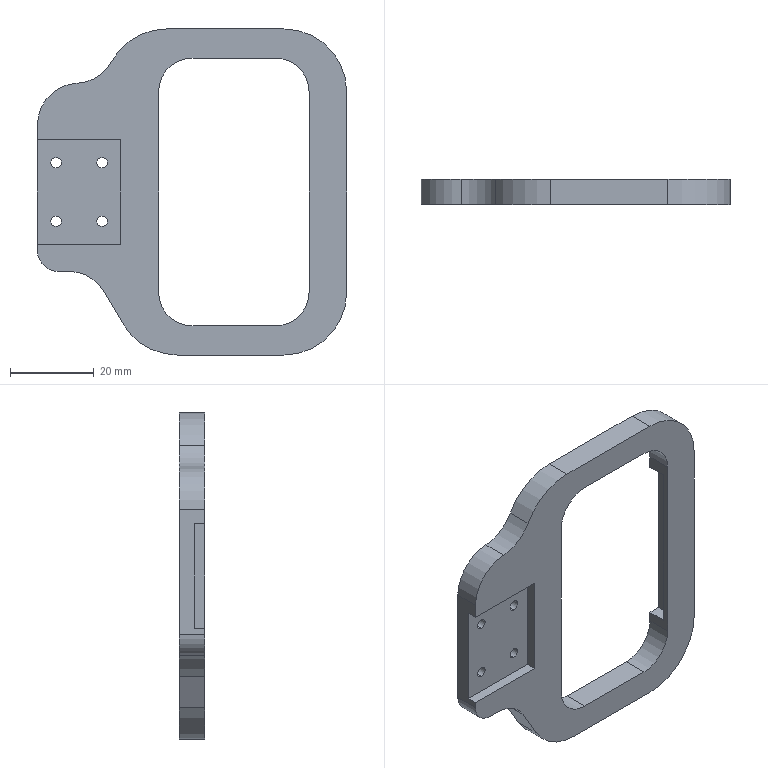Part | SolidWorks | features BaseBody 1, Cut 1, HoleWzd 1 | 1 solid | 44 faces | box 74 x 6 x 78 mm | volume 14123 mm3 | plane 24 | cylinder 20 | commonest cylinder face diameters 2.5 x8 16 x4 30 x4 20 x3 10 x1
STEP:
#1=CARTESIAN_POINT('',(1280.5,6.,-8.25));
#2=VERTEX_POINT('',#1);
#3=CARTESIAN_POINT('',(1280.5,6.,-5.75));
#4=VERTEX_POINT('',#3);
#5=CARTESIAN_POINT('',(1280.5,6.,-7.));
#6=DIRECTION('',(0.,1.,0.));
#7=DIRECTION('',(0.,0.,1.));
#8=AXIS2_PLACEMENT_3D('',#5,#6,#7);
#9=CIRCLE('',#8,1.25);
#10=EDGE_CURVE('',#2,#4,#9,.T.);
#11=ORIENTED_EDGE('',*,*,#10,.T.);
#12=CARTESIAN_POINT('',(1280.5,2.5,-5.75));
#13=VERTEX_POINT('',#12);
#14=CARTESIAN_POINT('',(1280.5,0.,-5.75));
#15=DIRECTION('',(0.,-1.,0.));
#16=VECTOR('',#15,1000.);
#17=LINE('',#14,#16);
#18=EDGE_CURVE('',#4,#13,#17,.T.);
#19=ORIENTED_EDGE('',*,*,#18,.T.);
#20=CARTESIAN_POINT('',(1280.5,2.5,-8.25));
#21=VERTEX_POINT('',#20);
#22=CARTESIAN_POINT('',(1280.5,2.5,-7.));
#23=DIRECTION('',(0.,-1.,0.));
#24=DIRECTION('',(0.,0.,-1.));
#25=AXIS2_PLACEMENT_3D('',#22,#23,#24);
#26=CIRCLE('',#25,1.25);
#27=EDGE_CURVE('',#13,#21,#26,.T.);
#28=ORIENTED_EDGE('',*,*,#27,.T.);
#29=CARTESIAN_POINT('',(1280.5,0.,-8.25));
#30=DIRECTION('',(0.,-1.,0.));
#31=VECTOR('',#30,1000.);
#32=LINE('',#29,#31);
#33=EDGE_CURVE('',#2,#21,#32,.T.);
#34=ORIENTED_EDGE('',*,*,#33,.F.);
#35=EDGE_LOOP('',(#11,#19,#28,#34));
#36=FACE_OUTER_BOUND('',#35,.T.);
#37=CARTESIAN_POINT('',(1280.5,0.,-7.));
#38=DIRECTION('',(0.,-1.,0.));
#39=DIRECTION('',(0.,0.,-1.));
#40=AXIS2_PLACEMENT_3D('',#37,#38,#39);
#41=CYLINDRICAL_SURFACE('',#40,1.25);
#42=ADVANCED_FACE('',(#36),#41,.F.);
#43=CARTESIAN_POINT('',(1269.5,6.,-8.25));
#44=VERTEX_POINT('',#43);
#45=CARTESIAN_POINT('',(1269.5,6.,-5.75));
#46=VERTEX_POINT('',#45);
#47=CARTESIAN_POINT('',(1269.5,6.,-7.));
#48=DIRECTION('',(0.,1.,0.));
#49=DIRECTION('',(0.,0.,1.));
#50=AXIS2_PLACEMENT_3D('',#47,#48,#49);
#51=CIRCLE('',#50,1.25);
#52=EDGE_CURVE('',#44,#46,#51,.T.);
#53=ORIENTED_EDGE('',*,*,#52,.T.);
#54=CARTESIAN_POINT('',(1269.5,2.5,-5.75));
#55=VERTEX_POINT('',#54);
#56=CARTESIAN_POINT('',(1269.5,0.,-5.75));
#57=DIRECTION('',(0.,-1.,0.));
#58=VECTOR('',#57,1000.);
#59=LINE('',#56,#58);
#60=EDGE_CURVE('',#46,#55,#59,.T.);
#61=ORIENTED_EDGE('',*,*,#60,.T.);
#62=CARTESIAN_POINT('',(1269.5,2.5,-8.25));
#63=VERTEX_POINT('',#62);
#64=CARTESIAN_POINT('',(1269.5,2.5,-7.));
#65=DIRECTION('',(0.,-1.,0.));
#66=DIRECTION('',(0.,0.,-1.));
#67=AXIS2_PLACEMENT_3D('',#64,#65,#66);
#68=CIRCLE('',#67,1.25);
#69=EDGE_CURVE('',#55,#63,#68,.T.);
#70=ORIENTED_EDGE('',*,*,#69,.T.);
#71=CARTESIAN_POINT('',(1269.5,0.,-8.25));
#72=DIRECTION('',(0.,-1.,0.));
#73=VECTOR('',#72,1000.);
#74=LINE('',#71,#73);
#75=EDGE_CURVE('',#44,#63,#74,.T.);
#76=ORIENTED_EDGE('',*,*,#75,.F.);
#77=EDGE_LOOP('',(#53,#61,#70,#76));
#78=FACE_OUTER_BOUND('',#77,.T.);
#79=CARTESIAN_POINT('',(1269.5,0.,-7.));
#80=DIRECTION('',(0.,-1.,0.));
#81=DIRECTION('',(0.,0.,-1.));
#82=AXIS2_PLACEMENT_3D('',#79,#80,#81);
#83=CYLINDRICAL_SURFACE('',#82,1.25);
#84=ADVANCED_FACE('',(#78),#83,.F.);
#85=CARTESIAN_POINT('',(1269.5,6.,5.75));
#86=VERTEX_POINT('',#85);
#87=CARTESIAN_POINT('',(1269.5,6.,8.25));
#88=VERTEX_POINT('',#87);
#89=CARTESIAN_POINT('',(1269.5,6.,7.));
#90=DIRECTION('',(0.,1.,0.));
#91=DIRECTION('',(0.,0.,1.));
#92=AXIS2_PLACEMENT_3D('',#89,#90,#91);
#93=CIRCLE('',#92,1.25);
#94=EDGE_CURVE('',#86,#88,#93,.T.);
#95=ORIENTED_EDGE('',*,*,#94,.T.);
#96=CARTESIAN_POINT('',(1269.5,2.5,8.25));
#97=VERTEX_POINT('',#96);
#98=CARTESIAN_POINT('',(1269.5,0.,8.25));
#99=DIRECTION('',(0.,-1.,0.));
#100=VECTOR('',#99,1000.);
#101=LINE('',#98,#100);
#102=EDGE_CURVE('',#88,#97,#101,.T.);
#103=ORIENTED_EDGE('',*,*,#102,.T.);
#104=CARTESIAN_POINT('',(1269.5,2.5,5.75));
#105=VERTEX_POINT('',#104);
#106=CARTESIAN_POINT('',(1269.5,2.5,7.));
#107=DIRECTION('',(0.,-1.,0.));
#108=DIRECTION('',(0.,0.,-1.));
#109=AXIS2_PLACEMENT_3D('',#106,#107,#108);
#110=CIRCLE('',#109,1.25);
#111=EDGE_CURVE('',#97,#105,#110,.T.);
#112=ORIENTED_EDGE('',*,*,#111,.T.);
#113=CARTESIAN_POINT('',(1269.5,0.,5.75));
#114=DIRECTION('',(0.,-1.,0.));
#115=VECTOR('',#114,1000.);
#116=LINE('',#113,#115);
#117=EDGE_CURVE('',#86,#105,#116,.T.);
#118=ORIENTED_EDGE('',*,*,#117,.F.);
#119=EDGE_LOOP('',(#95,#103,#112,#118));
#120=FACE_OUTER_BOUND('',#119,.T.);
#121=CARTESIAN_POINT('',(1269.5,0.,7.));
#122=DIRECTION('',(0.,-1.,0.));
#123=DIRECTION('',(0.,0.,-1.));
#124=AXIS2_PLACEMENT_3D('',#121,#122,#123);
#125=CYLINDRICAL_SURFACE('',#124,1.25);
#126=ADVANCED_FACE('',(#120),#125,.F.);
#127=CARTESIAN_POINT('',(1280.5,6.,5.75));
#128=VERTEX_POINT('',#127);
#129=CARTESIAN_POINT('',(1280.5,6.,8.25));
#130=VERTEX_POINT('',#129);
#131=CARTESIAN_POINT('',(1280.5,6.,7.));
#132=DIRECTION('',(0.,1.,0.));
#133=DIRECTION('',(0.,0.,1.));
#134=AXIS2_PLACEMENT_3D('',#131,#132,#133);
#135=CIRCLE('',#134,1.25);
#136=EDGE_CURVE('',#128,#130,#135,.T.);
#137=ORIENTED_EDGE('',*,*,#136,.T.);
#138=CARTESIAN_POINT('',(1280.5,2.5,8.25));
#139=VERTEX_POINT('',#138);
#140=CARTESIAN_POINT('',(1280.5,0.,8.25));
#141=DIRECTION('',(0.,-1.,0.));
#142=VECTOR('',#141,1000.);
#143=LINE('',#140,#142);
#144=EDGE_CURVE('',#130,#139,#143,.T.);
#145=ORIENTED_EDGE('',*,*,#144,.T.);
#146=CARTESIAN_POINT('',(1280.5,2.5,5.75));
#147=VERTEX_POINT('',#146);
#148=CARTESIAN_POINT('',(1280.5,2.5,7.));
#149=DIRECTION('',(0.,-1.,0.));
#150=DIRECTION('',(0.,0.,-1.));
#151=AXIS2_PLACEMENT_3D('',#148,#149,#150);
#152=CIRCLE('',#151,1.25);
#153=EDGE_CURVE('',#139,#147,#152,.T.);
#154=ORIENTED_EDGE('',*,*,#153,.T.);
#155=CARTESIAN_POINT('',(1280.5,0.,5.75));
#156=DIRECTION('',(0.,-1.,0.));
#157=VECTOR('',#156,1000.);
#158=LINE('',#155,#157);
#159=EDGE_CURVE('',#128,#147,#158,.T.);
#160=ORIENTED_EDGE('',*,*,#159,.F.);
#161=EDGE_LOOP('',(#137,#145,#154,#160));
#162=FACE_OUTER_BOUND('',#161,.T.);
#163=CARTESIAN_POINT('',(1280.5,0.,7.));
#164=DIRECTION('',(0.,-1.,0.));
#165=DIRECTION('',(0.,0.,-1.));
#166=AXIS2_PLACEMENT_3D('',#163,#164,#165);
#167=CYLINDRICAL_SURFACE('',#166,1.25);
#168=ADVANCED_FACE('',(#162),#167,.F.);
#169=CARTESIAN_POINT('',(1285.,0.,12.5));
#170=VERTEX_POINT('',#169);
#171=CARTESIAN_POINT('',(1265.,0.,12.5));
#172=VERTEX_POINT('',#171);
#173=CARTESIAN_POINT('',(1265.,0.,12.5));
#174=DIRECTION('',(-1.,0.,0.));
#175=VECTOR('',#174,1000.);
#176=LINE('',#173,#175);
#177=EDGE_CURVE('',#170,#172,#176,.T.);
#178=ORIENTED_EDGE('',*,*,#177,.F.);
#179=CARTESIAN_POINT('',(1285.,0.,-12.5));
#180=VERTEX_POINT('',#179);
#181=CARTESIAN_POINT('',(1285.,0.,12.5));
#182=DIRECTION('',(0.,0.,1.));
#183=VECTOR('',#182,1000.);
#184=LINE('',#181,#183);
#185=EDGE_CURVE('',#180,#170,#184,.T.);
#186=ORIENTED_EDGE('',*,*,#185,.F.);
#187=CARTESIAN_POINT('',(1265.,0.,-12.5));
#188=VERTEX_POINT('',#187);
#189=CARTESIAN_POINT('',(1265.,0.,-12.5));
#190=DIRECTION('',(1.,0.,0.));
#191=VECTOR('',#190,1000.);
#192=LINE('',#189,#191);
#193=EDGE_CURVE('',#188,#180,#192,.T.);
#194=ORIENTED_EDGE('',*,*,#193,.F.);
#195=CARTESIAN_POINT('',(1265.,0.,-13.995));
#196=VERTEX_POINT('',#195);
#197=CARTESIAN_POINT('',(1265.,0.,0.));
#198=DIRECTION('',(0.,0.,-1.));
#199=VECTOR('',#198,1000.);
#200=LINE('',#197,#199);
#201=EDGE_CURVE('',#188,#196,#200,.T.);
#202=ORIENTED_EDGE('',*,*,#201,.T.);
#203=CARTESIAN_POINT('',(1270.,0.,-18.995));
#204=VERTEX_POINT('',#203);
#205=CARTESIAN_POINT('',(1270.,0.,-13.995));
#206=DIRECTION('',(0.,-1.,0.));
#207=DIRECTION('',(0.,0.,-1.));
#208=AXIS2_PLACEMENT_3D('',#205,#206,#207);
#209=CIRCLE('',#208,5.);
#210=EDGE_CURVE('',#196,#204,#209,.T.);
#211=ORIENTED_EDGE('',*,*,#210,.T.);
#212=CARTESIAN_POINT('',(1272.447,0.,-18.995));
#213=VERTEX_POINT('',#212);
#214=CARTESIAN_POINT('',(0.,0.,-18.995));
#215=DIRECTION('',(1.,0.,0.));
#216=VECTOR('',#215,1000.);
#217=LINE('',#214,#216);
#218=EDGE_CURVE('',#204,#213,#217,.T.);
#219=ORIENTED_EDGE('',*,*,#218,.T.);
#220=CARTESIAN_POINT('',(1281.087,0.,-23.96));
#221=VERTEX_POINT('',#220);
#222=CARTESIAN_POINT('',(1272.447,0.,-28.995));
#223=DIRECTION('',(0.,1.,0.));
#224=DIRECTION('',(0.,0.,1.));
#225=AXIS2_PLACEMENT_3D('',#222,#223,#224);
#226=CIRCLE('',#225,10.);
#227=EDGE_CURVE('',#213,#221,#226,.T.);
#228=ORIENTED_EDGE('',*,*,#227,.T.);
#229=CARTESIAN_POINT('',(1285.513,0.,-31.554));
#230=VERTEX_POINT('',#229);
#231=CARTESIAN_POINT('',(1281.087,0.,-23.96));
#232=DIRECTION('',(0.5036,0.,-0.8639));
#233=VECTOR('',#232,1000.);
#234=LINE('',#231,#233);
#235=EDGE_CURVE('',#221,#230,#234,.T.);
#236=ORIENTED_EDGE('',*,*,#235,.T.);
#237=CARTESIAN_POINT('',(1298.473,0.,-39.));
#238=VERTEX_POINT('',#237);
#239=CARTESIAN_POINT('',(1298.473,0.,-24.));
#240=DIRECTION('',(0.,-1.,0.));
#241=DIRECTION('',(0.,0.,1.));
#242=AXIS2_PLACEMENT_3D('',#239,#240,#241);
#243=CIRCLE('',#242,15.);
#244=EDGE_CURVE('',#230,#238,#243,.T.);
#245=ORIENTED_EDGE('',*,*,#244,.T.);
#246=CARTESIAN_POINT('',(1324.,0.,-39.));
#247=VERTEX_POINT('',#246);
#248=CARTESIAN_POINT('',(0.,0.,-39.));
#249=DIRECTION('',(1.,0.,0.));
#250=VECTOR('',#249,1000.);
#251=LINE('',#248,#250);
#252=EDGE_CURVE('',#238,#247,#251,.T.);
#253=ORIENTED_EDGE('',*,*,#252,.T.);
#254=CARTESIAN_POINT('',(1339.,0.,-24.));
#255=VERTEX_POINT('',#254);
#256=CARTESIAN_POINT('',(1324.,0.,-24.));
#257=DIRECTION('',(0.,-1.,0.));
#258=DIRECTION('',(0.,0.,1.));
#259=AXIS2_PLACEMENT_3D('',#256,#257,#258);
#260=CIRCLE('',#259,15.);
#261=EDGE_CURVE('',#247,#255,#260,.T.);
#262=ORIENTED_EDGE('',*,*,#261,.T.);
#263=CARTESIAN_POINT('',(1339.,0.,24.));
#264=VERTEX_POINT('',#263);
#265=CARTESIAN_POINT('',(1339.,0.,0.));
#266=DIRECTION('',(0.,0.,1.));
#267=VECTOR('',#266,1000.);
#268=LINE('',#265,#267);
#269=EDGE_CURVE('',#255,#264,#268,.T.);
#270=ORIENTED_EDGE('',*,*,#269,.T.);
#271=CARTESIAN_POINT('',(1324.,0.,39.));
#272=VERTEX_POINT('',#271);
#273=CARTESIAN_POINT('',(1324.,0.,24.));
#274=DIRECTION('',(0.,-1.,0.));
#275=DIRECTION('',(0.,0.,1.));
#276=AXIS2_PLACEMENT_3D('',#273,#274,#275);
#277=CIRCLE('',#276,15.);
#278=EDGE_CURVE('',#264,#272,#277,.T.);
#279=ORIENTED_EDGE('',*,*,#278,.T.);
#280=CARTESIAN_POINT('',(1295.928,0.,39.));
#281=VERTEX_POINT('',#280);
#282=CARTESIAN_POINT('',(0.,0.,39.));
#283=DIRECTION('',(-1.,0.,0.));
#284=VECTOR('',#283,1000.);
#285=LINE('',#282,#284);
#286=EDGE_CURVE('',#272,#281,#285,.T.);
#287=ORIENTED_EDGE('',*,*,#286,.T.);
#288=CARTESIAN_POINT('',(1282.769,0.,31.2));
#289=VERTEX_POINT('',#288);
#290=CARTESIAN_POINT('',(1295.928,0.,24.));
#291=DIRECTION('',(0.,-1.,0.));
#292=DIRECTION('',(0.,0.,1.));
#293=AXIS2_PLACEMENT_3D('',#290,#291,#292);
#294=CIRCLE('',#293,15.);
#295=EDGE_CURVE('',#281,#289,#294,.T.);
#296=ORIENTED_EDGE('',*,*,#295,.T.);
#297=CARTESIAN_POINT('',(1274.498,0.,26.013));
#298=VERTEX_POINT('',#297);
#299=CARTESIAN_POINT('',(1273.997,0.,36.));
#300=DIRECTION('',(0.,1.,0.));
#301=DIRECTION('',(0.,0.,1.));
#302=AXIS2_PLACEMENT_3D('',#299,#300,#301);
#303=CIRCLE('',#302,10.);
#304=EDGE_CURVE('',#289,#298,#303,.T.);
#305=ORIENTED_EDGE('',*,*,#304,.T.);
#306=CARTESIAN_POINT('',(1265.,0.,16.025));
#307=VERTEX_POINT('',#306);
#308=CARTESIAN_POINT('',(1275.,0.,16.025));
#309=DIRECTION('',(0.,-1.,0.));
#310=DIRECTION('',(0.,0.,-1.));
#311=AXIS2_PLACEMENT_3D('',#308,#309,#310);
#312=CIRCLE('',#311,10.);
#313=EDGE_CURVE('',#298,#307,#312,.T.);
#314=ORIENTED_EDGE('',*,*,#313,.T.);
#315=CARTESIAN_POINT('',(1265.,0.,0.));
#316=DIRECTION('',(0.,0.,-1.));
#317=VECTOR('',#316,1000.);
#318=LINE('',#315,#317);
#319=EDGE_CURVE('',#307,#172,#318,.T.);
#320=ORIENTED_EDGE('',*,*,#319,.T.);
#321=EDGE_LOOP('',(#178,#186,#194,#202,#211,#219,#228,#236,#245,#253,#262,#270,#279,#287,#296,#305,#314,#320));
#322=FACE_OUTER_BOUND('',#321,.T.);
#323=CARTESIAN_POINT('',(1330.,0.,-24.));
#324=VERTEX_POINT('',#323);
#325=CARTESIAN_POINT('',(1322.,0.,-32.));
#326=VERTEX_POINT('',#325);
#327=CARTESIAN_POINT('',(1322.,0.,-24.));
#328=DIRECTION('',(0.,1.,0.));
#329=DIRECTION('',(0.,0.,1.));
#330=AXIS2_PLACEMENT_3D('',#327,#328,#329);
#331=CIRCLE('',#330,8.);
#332=EDGE_CURVE('',#324,#326,#331,.T.);
#333=ORIENTED_EDGE('',*,*,#332,.T.);
#334=CARTESIAN_POINT('',(1302.,0.,-32.));
#335=VERTEX_POINT('',#334);
#336=CARTESIAN_POINT('',(0.,0.,-32.));
#337=DIRECTION('',(-1.,0.,0.));
#338=VECTOR('',#337,1000.);
#339=LINE('',#336,#338);
#340=EDGE_CURVE('',#326,#335,#339,.T.);
#341=ORIENTED_EDGE('',*,*,#340,.T.);
#342=CARTESIAN_POINT('',(1294.,0.,-24.));
#343=VERTEX_POINT('',#342);
#344=CARTESIAN_POINT('',(1302.,0.,-24.));
#345=DIRECTION('',(0.,1.,0.));
#346=DIRECTION('',(0.,0.,1.));
#347=AXIS2_PLACEMENT_3D('',#344,#345,#346);
#348=CIRCLE('',#347,8.);
#349=EDGE_CURVE('',#335,#343,#348,.T.);
#350=ORIENTED_EDGE('',*,*,#349,.T.);
#351=CARTESIAN_POINT('',(1294.,0.,24.));
#352=VERTEX_POINT('',#351);
#353=CARTESIAN_POINT('',(1294.,0.,0.));
#354=DIRECTION('',(0.,0.,1.));
#355=VECTOR('',#354,1000.);
#356=LINE('',#353,#355);
#357=EDGE_CURVE('',#343,#352,#356,.T.);
#358=ORIENTED_EDGE('',*,*,#357,.T.);
#359=CARTESIAN_POINT('',(1302.,0.,32.));
#360=VERTEX_POINT('',#359);
#361=CARTESIAN_POINT('',(1302.,0.,24.));
#362=DIRECTION('',(0.,1.,0.));
#363=DIRECTION('',(0.,0.,1.));
#364=AXIS2_PLACEMENT_3D('',#361,#362,#363);
#365=CIRCLE('',#364,8.);
#366=EDGE_CURVE('',#352,#360,#365,.T.);
#367=ORIENTED_EDGE('',*,*,#366,.T.);
#368=CARTESIAN_POINT('',(1322.,0.,32.));
#369=VERTEX_POINT('',#368);
#370=CARTESIAN_POINT('',(0.,0.,32.));
#371=DIRECTION('',(1.,0.,0.));
#372=VECTOR('',#371,1000.);
#373=LINE('',#370,#372);
#374=EDGE_CURVE('',#360,#369,#373,.T.);
#375=ORIENTED_EDGE('',*,*,#374,.T.);
#376=CARTESIAN_POINT('',(1330.,0.,24.));
#377=VERTEX_POINT('',#376);
#378=CARTESIAN_POINT('',(1322.,0.,24.));
#379=DIRECTION('',(0.,1.,0.));
#380=DIRECTION('',(0.,0.,1.));
#381=AXIS2_PLACEMENT_3D('',#378,#379,#380);
#382=CIRCLE('',#381,8.);
#383=EDGE_CURVE('',#369,#377,#382,.T.);
#384=ORIENTED_EDGE('',*,*,#383,.T.);
#385=CARTESIAN_POINT('',(1330.,0.,0.));
#386=DIRECTION('',(0.,0.,-1.));
#387=VECTOR('',#386,1000.);
#388=LINE('',#385,#387);
#389=EDGE_CURVE('',#377,#324,#388,.T.);
#390=ORIENTED_EDGE('',*,*,#389,.T.);
#391=EDGE_LOOP('',(#333,#341,#350,#358,#367,#375,#384,#390));
#392=FACE_BOUND('',#391,.T.);
#393=CARTESIAN_POINT('',(0.,0.,0.));
#394=DIRECTION('',(0.,-1.,0.));
#395=DIRECTION('',(0.,0.,-1.));
#396=AXIS2_PLACEMENT_3D('',#393,#394,#395);
#397=PLANE('',#396);
#398=ADVANCED_FACE('',(#322,#392),#397,.T.);
#399=CARTESIAN_POINT('',(1302.,6.,-32.));
#400=VERTEX_POINT('',#399);
#401=CARTESIAN_POINT('',(1322.,6.,-32.));
#402=VERTEX_POINT('',#401);
#403=CARTESIAN_POINT('',(1302.,6.,-32.));
#404=DIRECTION('',(1.,0.,0.));
#405=VECTOR('',#404,1000.);
#406=LINE('',#403,#405);
#407=EDGE_CURVE('',#400,#402,#406,.T.);
#408=ORIENTED_EDGE('',*,*,#407,.F.);
#409=CARTESIAN_POINT('',(1302.,0.,-32.));
#410=DIRECTION('',(0.,1.,0.));
#411=VECTOR('',#410,1000.);
#412=LINE('',#409,#411);
#413=EDGE_CURVE('',#335,#400,#412,.T.);
#414=ORIENTED_EDGE('',*,*,#413,.F.);
#415=ORIENTED_EDGE('',*,*,#340,.F.);
#416=CARTESIAN_POINT('',(1322.,0.,-32.));
#417=DIRECTION('',(0.,-1.,0.));
#418=VECTOR('',#417,1000.);
#419=LINE('',#416,#418);
#420=EDGE_CURVE('',#402,#326,#419,.T.);
#421=ORIENTED_EDGE('',*,*,#420,.F.);
#422=EDGE_LOOP('',(#408,#414,#415,#421));
#423=FACE_OUTER_BOUND('',#422,.T.);
#424=CARTESIAN_POINT('',(1302.,0.,-32.));
#425=DIRECTION('',(0.,0.,-1.));
#426=DIRECTION('',(-1.,0.,0.));
#427=AXIS2_PLACEMENT_3D('',#424,#425,#426);
#428=PLANE('',#427);
#429=ADVANCED_FACE('',(#423),#428,.F.);
#430=CARTESIAN_POINT('',(1330.,6.,-24.));
#431=VERTEX_POINT('',#430);
#432=CARTESIAN_POINT('',(1322.,6.,-24.));
#433=DIRECTION('',(0.,-1.,0.));
#434=DIRECTION('',(0.,0.,1.));
#435=AXIS2_PLACEMENT_3D('',#432,#433,#434);
#436=CIRCLE('',#435,8.);
#437=EDGE_CURVE('',#402,#431,#436,.T.);
#438=ORIENTED_EDGE('',*,*,#437,.F.);
#439=ORIENTED_EDGE('',*,*,#420,.T.);
#440=ORIENTED_EDGE('',*,*,#332,.F.);
#441=CARTESIAN_POINT('',(1330.,0.,-24.));
#442=DIRECTION('',(0.,-1.,0.));
#443=VECTOR('',#442,1000.);
#444=LINE('',#441,#443);
#445=EDGE_CURVE('',#431,#324,#444,.T.);
#446=ORIENTED_EDGE('',*,*,#445,.F.);
#447=EDGE_LOOP('',(#438,#439,#440,#446));
#448=FACE_OUTER_BOUND('',#447,.T.);
#449=CARTESIAN_POINT('',(1322.,0.,-24.));
#450=DIRECTION('',(0.,1.,0.));
#451=DIRECTION('',(0.,0.,1.));
#452=AXIS2_PLACEMENT_3D('',#449,#450,#451);
#453=CYLINDRICAL_SURFACE('',#452,8.);
#454=ADVANCED_FACE('',(#448),#453,.F.);
#455=CARTESIAN_POINT('',(1330.,6.,-21.548));
#456=VERTEX_POINT('',#455);
#457=CARTESIAN_POINT('',(1330.,6.,-24.));
#458=DIRECTION('',(0.,0.,1.));
#459=VECTOR('',#458,1000.);
#460=LINE('',#457,#459);
#461=EDGE_CURVE('',#431,#456,#460,.T.);
#462=ORIENTED_EDGE('',*,*,#461,.F.);
#463=ORIENTED_EDGE('',*,*,#445,.T.);
#464=ORIENTED_EDGE('',*,*,#389,.F.);
#465=CARTESIAN_POINT('',(1330.,6.,24.));
#466=VERTEX_POINT('',#465);
#467=CARTESIAN_POINT('',(1330.,0.,24.));
#468=DIRECTION('',(0.,-1.,0.));
#469=VECTOR('',#468,1000.);
#470=LINE('',#467,#469);
#471=EDGE_CURVE('',#466,#377,#470,.T.);
#472=ORIENTED_EDGE('',*,*,#471,.F.);
#473=CARTESIAN_POINT('',(1330.,6.,21.019));
#474=VERTEX_POINT('',#473);
#475=CARTESIAN_POINT('',(1330.,6.,-24.));
#476=DIRECTION('',(0.,0.,1.));
#477=VECTOR('',#476,1000.);
#478=LINE('',#475,#477);
#479=EDGE_CURVE('',#474,#466,#478,.T.);
#480=ORIENTED_EDGE('',*,*,#479,.F.);
#481=CARTESIAN_POINT('',(1330.,1.5,21.019));
#482=VERTEX_POINT('',#481);
#483=CARTESIAN_POINT('',(1330.,0.,21.019));
#484=DIRECTION('',(0.,1.,0.));
#485=VECTOR('',#484,1000.);
#486=LINE('',#483,#485);
#487=EDGE_CURVE('',#482,#474,#486,.T.);
#488=ORIENTED_EDGE('',*,*,#487,.F.);
#489=CARTESIAN_POINT('',(1330.,1.5,-21.548));
#490=VERTEX_POINT('',#489);
#491=CARTESIAN_POINT('',(1330.,1.5,-24.));
#492=DIRECTION('',(0.,0.,1.));
#493=VECTOR('',#492,1000.);
#494=LINE('',#491,#493);
#495=EDGE_CURVE('',#490,#482,#494,.T.);
#496=ORIENTED_EDGE('',*,*,#495,.F.);
#497=CARTESIAN_POINT('',(1330.,0.,-21.548));
#498=DIRECTION('',(0.,-1.,0.));
#499=VECTOR('',#498,1000.);
#500=LINE('',#497,#499);
#501=EDGE_CURVE('',#456,#490,#500,.T.);
#502=ORIENTED_EDGE('',*,*,#501,.F.);
#503=EDGE_LOOP('',(#462,#463,#464,#472,#480,#488,#496,#502));
#504=FACE_OUTER_BOUND('',#503,.T.);
#505=CARTESIAN_POINT('',(1330.,0.,-24.));
#506=DIRECTION('',(1.,0.,0.));
#507=DIRECTION('',(0.,0.,-1.));
#508=AXIS2_PLACEMENT_3D('',#505,#506,#507);
#509=PLANE('',#508);
#510=ADVANCED_FACE('',(#504),#509,.F.);
#511=CARTESIAN_POINT('',(1322.,6.,32.));
#512=VERTEX_POINT('',#511);
#513=CARTESIAN_POINT('',(1322.,6.,24.));
#514=DIRECTION('',(0.,-1.,0.));
#515=DIRECTION('',(0.,0.,1.));
#516=AXIS2_PLACEMENT_3D('',#513,#514,#515);
#517=CIRCLE('',#516,8.);
#518=EDGE_CURVE('',#466,#512,#517,.T.);
#519=ORIENTED_EDGE('',*,*,#518,.F.);
#520=ORIENTED_EDGE('',*,*,#471,.T.);
#521=ORIENTED_EDGE('',*,*,#383,.F.);
#522=CARTESIAN_POINT('',(1322.,0.,32.));
#523=DIRECTION('',(0.,-1.,0.));
#524=VECTOR('',#523,1000.);
#525=LINE('',#522,#524);
#526=EDGE_CURVE('',#512,#369,#525,.T.);
#527=ORIENTED_EDGE('',*,*,#526,.F.);
#528=EDGE_LOOP('',(#519,#520,#521,#527));
#529=FACE_OUTER_BOUND('',#528,.T.);
#530=CARTESIAN_POINT('',(1322.,0.,24.));
#531=DIRECTION('',(0.,1.,0.));
#532=DIRECTION('',(0.,0.,1.));
#533=AXIS2_PLACEMENT_3D('',#530,#531,#532);
#534=CYLINDRICAL_SURFACE('',#533,8.);
#535=ADVANCED_FACE('',(#529),#534,.F.);
#536=CARTESIAN_POINT('',(1302.,6.,32.));
#537=VERTEX_POINT('',#536);
#538=CARTESIAN_POINT('',(1322.,6.,32.));
#539=DIRECTION('',(-1.,0.,0.));
#540=VECTOR('',#539,1000.);
#541=LINE('',#538,#540);
#542=EDGE_CURVE('',#512,#537,#541,.T.);
#543=ORIENTED_EDGE('',*,*,#542,.F.);
#544=ORIENTED_EDGE('',*,*,#526,.T.);
#545=ORIENTED_EDGE('',*,*,#374,.F.);
#546=CARTESIAN_POINT('',(1302.,0.,32.));
#547=DIRECTION('',(0.,-1.,0.));
#548=VECTOR('',#547,1000.);
#549=LINE('',#546,#548);
#550=EDGE_CURVE('',#537,#360,#549,.T.);
#551=ORIENTED_EDGE('',*,*,#550,.F.);
#552=EDGE_LOOP('',(#543,#544,#545,#551));
#553=FACE_OUTER_BOUND('',#552,.T.);
#554=CARTESIAN_POINT('',(1322.,0.,32.));
#555=DIRECTION('',(0.,0.,1.));
#556=DIRECTION('',(1.,0.,0.));
#557=AXIS2_PLACEMENT_3D('',#554,#555,#556);
#558=PLANE('',#557);
#559=ADVANCED_FACE('',(#553),#558,.F.);
#560=CARTESIAN_POINT('',(1294.,6.,24.));
#561=VERTEX_POINT('',#560);
#562=CARTESIAN_POINT('',(1302.,6.,24.));
#563=DIRECTION('',(0.,-1.,0.));
#564=DIRECTION('',(0.,0.,1.));
#565=AXIS2_PLACEMENT_3D('',#562,#563,#564);
#566=CIRCLE('',#565,8.);
#567=EDGE_CURVE('',#537,#561,#566,.T.);
#568=ORIENTED_EDGE('',*,*,#567,.F.);
#569=ORIENTED_EDGE('',*,*,#550,.T.);
#570=ORIENTED_EDGE('',*,*,#366,.F.);
#571=CARTESIAN_POINT('',(1294.,0.,24.));
#572=DIRECTION('',(0.,-1.,0.));
#573=VECTOR('',#572,1000.);
#574=LINE('',#571,#573);
#575=EDGE_CURVE('',#561,#352,#574,.T.);
#576=ORIENTED_EDGE('',*,*,#575,.F.);
#577=EDGE_LOOP('',(#568,#569,#570,#576));
#578=FACE_OUTER_BOUND('',#577,.T.);
#579=CARTESIAN_POINT('',(1302.,0.,24.));
#580=DIRECTION('',(0.,1.,0.));
#581=DIRECTION('',(0.,0.,1.));
#582=AXIS2_PLACEMENT_3D('',#579,#580,#581);
#583=CYLINDRICAL_SURFACE('',#582,8.);
#584=ADVANCED_FACE('',(#578),#583,.F.);
#585=CARTESIAN_POINT('',(1294.,6.,21.019));
#586=VERTEX_POINT('',#585);
#587=CARTESIAN_POINT('',(1294.,6.,24.));
#588=DIRECTION('',(0.,0.,-1.));
#589=VECTOR('',#588,1000.);
#590=LINE('',#587,#589);
#591=EDGE_CURVE('',#561,#586,#590,.T.);
#592=ORIENTED_EDGE('',*,*,#591,.F.);
#593=ORIENTED_EDGE('',*,*,#575,.T.);
#594=ORIENTED_EDGE('',*,*,#357,.F.);
#595=CARTESIAN_POINT('',(1294.,6.,-24.));
#596=VERTEX_POINT('',#595);
#597=CARTESIAN_POINT('',(1294.,0.,-24.));
#598=DIRECTION('',(0.,-1.,0.));
#599=VECTOR('',#598,1000.);
#600=LINE('',#597,#599);
#601=EDGE_CURVE('',#596,#343,#600,.T.);
#602=ORIENTED_EDGE('',*,*,#601,.F.);
#603=CARTESIAN_POINT('',(1294.,6.,-21.548));
#604=VERTEX_POINT('',#603);
#605=CARTESIAN_POINT('',(1294.,6.,24.));
#606=DIRECTION('',(0.,0.,-1.));
#607=VECTOR('',#606,1000.);
#608=LINE('',#605,#607);
#609=EDGE_CURVE('',#604,#596,#608,.T.);
#610=ORIENTED_EDGE('',*,*,#609,.F.);
#611=CARTESIAN_POINT('',(1294.,1.5,-21.548));
#612=VERTEX_POINT('',#611);
#613=CARTESIAN_POINT('',(1294.,0.,-21.548));
#614=DIRECTION('',(0.,1.,0.));
#615=VECTOR('',#614,1000.);
#616=LINE('',#613,#615);
#617=EDGE_CURVE('',#612,#604,#616,.T.);
#618=ORIENTED_EDGE('',*,*,#617,.F.);
#619=CARTESIAN_POINT('',(1294.,1.5,21.019));
#620=VERTEX_POINT('',#619);
#621=CARTESIAN_POINT('',(1294.,1.5,24.));
#622=DIRECTION('',(0.,0.,-1.));
#623=VECTOR('',#622,1000.);
#624=LINE('',#621,#623);
#625=EDGE_CURVE('',#620,#612,#624,.T.);
#626=ORIENTED_EDGE('',*,*,#625,.F.);
#627=CARTESIAN_POINT('',(1294.,0.,21.019));
#628=DIRECTION('',(0.,-1.,0.));
#629=VECTOR('',#628,1000.);
#630=LINE('',#627,#629);
#631=EDGE_CURVE('',#586,#620,#630,.T.);
#632=ORIENTED_EDGE('',*,*,#631,.F.);
#633=EDGE_LOOP('',(#592,#593,#594,#602,#610,#618,#626,#632));
#634=FACE_OUTER_BOUND('',#633,.T.);
#635=CARTESIAN_POINT('',(1294.,0.,24.));
#636=DIRECTION('',(-1.,0.,0.));
#637=DIRECTION('',(0.,0.,1.));
#638=AXIS2_PLACEMENT_3D('',#635,#636,#637);
#639=PLANE('',#638);
#640=ADVANCED_FACE('',(#634),#639,.F.);
#641=CARTESIAN_POINT('',(1302.,6.,-24.));
#642=DIRECTION('',(0.,-1.,0.));
#643=DIRECTION('',(0.,0.,1.));
#644=AXIS2_PLACEMENT_3D('',#641,#642,#643);
#645=CIRCLE('',#644,8.);
#646=EDGE_CURVE('',#596,#400,#645,.T.);
#647=ORIENTED_EDGE('',*,*,#646,.F.);
#648=ORIENTED_EDGE('',*,*,#601,.T.);
#649=ORIENTED_EDGE('',*,*,#349,.F.);
#650=ORIENTED_EDGE('',*,*,#413,.T.);
#651=EDGE_LOOP('',(#647,#648,#649,#650));
#652=FACE_OUTER_BOUND('',#651,.T.);
#653=CARTESIAN_POINT('',(1302.,0.,-24.));
#654=DIRECTION('',(0.,1.,0.));
#655=DIRECTION('',(0.,0.,1.));
#656=AXIS2_PLACEMENT_3D('',#653,#654,#655);
#657=CYLINDRICAL_SURFACE('',#656,8.);
#658=ADVANCED_FACE('',(#652),#657,.F.);
#659=CARTESIAN_POINT('',(1265.,2.5,12.5));
#660=VERTEX_POINT('',#659);
#661=CARTESIAN_POINT('',(1265.,2.5,-12.5));
#662=VERTEX_POINT('',#661);
#663=CARTESIAN_POINT('',(1265.,2.5,12.5));
#664=DIRECTION('',(0.,0.,-1.));
#665=VECTOR('',#664,1000.);
#666=LINE('',#663,#665);
#667=EDGE_CURVE('',#660,#662,#666,.T.);
#668=ORIENTED_EDGE('',*,*,#667,.F.);
#669=CARTESIAN_POINT('',(1265.,2.5,12.5));
#670=DIRECTION('',(0.,-1.,0.));
#671=VECTOR('',#670,1000.);
#672=LINE('',#669,#671);
#673=EDGE_CURVE('',#660,#172,#672,.T.);
#674=ORIENTED_EDGE('',*,*,#673,.T.);
#675=ORIENTED_EDGE('',*,*,#319,.F.);
#676=CARTESIAN_POINT('',(1265.,6.,16.025));
#677=VERTEX_POINT('',#676);
#678=CARTESIAN_POINT('',(1265.,0.,16.025));
#679=DIRECTION('',(0.,-1.,0.));
#680=VECTOR('',#679,1000.);
#681=LINE('',#678,#680);
#682=EDGE_CURVE('',#677,#307,#681,.T.);
#683=ORIENTED_EDGE('',*,*,#682,.F.);
#684=CARTESIAN_POINT('',(1265.,6.,-13.995));
#685=VERTEX_POINT('',#684);
#686=CARTESIAN_POINT('',(1265.,6.,-18.995));
#687=DIRECTION('',(0.,0.,1.));
#688=VECTOR('',#687,1000.);
#689=LINE('',#686,#688);
#690=EDGE_CURVE('',#685,#677,#689,.T.);
#691=ORIENTED_EDGE('',*,*,#690,.F.);
#692=CARTESIAN_POINT('',(1265.,0.,-13.995));
#693=DIRECTION('',(0.,1.,0.));
#694=VECTOR('',#693,1000.);
#695=LINE('',#692,#694);
#696=EDGE_CURVE('',#196,#685,#695,.T.);
#697=ORIENTED_EDGE('',*,*,#696,.F.);
#698=ORIENTED_EDGE('',*,*,#201,.F.);
#699=CARTESIAN_POINT('',(1265.,2.5,-12.5));
#700=DIRECTION('',(0.,-1.,0.));
#701=VECTOR('',#700,1000.);
#702=LINE('',#699,#701);
#703=EDGE_CURVE('',#662,#188,#702,.T.);
#704=ORIENTED_EDGE('',*,*,#703,.F.);
#705=EDGE_LOOP('',(#668,#674,#675,#683,#691,#697,#698,#704));
#706=FACE_OUTER_BOUND('',#705,.T.);
#707=CARTESIAN_POINT('',(1265.,0.,-18.995));
#708=DIRECTION('',(1.,0.,0.));
#709=DIRECTION('',(0.,0.,-1.));
#710=AXIS2_PLACEMENT_3D('',#707,#708,#709);
#711=PLANE('',#710);
#712=ADVANCED_FACE('',(#706),#711,.F.);
#713=ORIENTED_EDGE('',*,*,#313,.F.);
#714=CARTESIAN_POINT('',(1274.498,6.,26.013));
#715=VERTEX_POINT('',#714);
#716=CARTESIAN_POINT('',(1274.498,-12.631,26.013));
#717=DIRECTION('',(0.,1.,0.));
#718=VECTOR('',#717,1000.);
#719=LINE('',#716,#718);
#720=EDGE_CURVE('',#298,#715,#719,.T.);
#721=ORIENTED_EDGE('',*,*,#720,.T.);
#722=CARTESIAN_POINT('',(1275.,6.,16.025));
#723=DIRECTION('',(0.,-1.,0.));
#724=DIRECTION('',(0.,0.,-1.));
#725=AXIS2_PLACEMENT_3D('',#722,#723,#724);
#726=CIRCLE('',#725,10.);
#727=EDGE_CURVE('',#715,#677,#726,.T.);
#728=ORIENTED_EDGE('',*,*,#727,.T.);
#729=ORIENTED_EDGE('',*,*,#682,.T.);
#730=EDGE_LOOP('',(#713,#721,#728,#729));
#731=FACE_OUTER_BOUND('',#730,.T.);
#732=CARTESIAN_POINT('',(1275.,-12.631,16.025));
#733=DIRECTION('',(0.,-1.,0.));
#734=DIRECTION('',(0.,0.,-1.));
#735=AXIS2_PLACEMENT_3D('',#732,#733,#734);
#736=CYLINDRICAL_SURFACE('',#735,10.);
#737=ADVANCED_FACE('',(#731),#736,.T.);
#738=CARTESIAN_POINT('',(1282.769,6.,31.2));
#739=VERTEX_POINT('',#738);
#740=CARTESIAN_POINT('',(1282.769,0.,31.2));
#741=DIRECTION('',(0.,-1.,0.));
#742=VECTOR('',#741,1000.);
#743=LINE('',#740,#742);
#744=EDGE_CURVE('',#739,#289,#743,.T.);
#745=ORIENTED_EDGE('',*,*,#744,.F.);
#746=CARTESIAN_POINT('',(1273.997,6.,36.));
#747=DIRECTION('',(0.,-1.,0.));
#748=DIRECTION('',(0.,0.,1.));
#749=AXIS2_PLACEMENT_3D('',#746,#747,#748);
#750=CIRCLE('',#749,10.);
#751=EDGE_CURVE('',#715,#739,#750,.T.);
#752=ORIENTED_EDGE('',*,*,#751,.F.);
#753=ORIENTED_EDGE('',*,*,#720,.F.);
#754=ORIENTED_EDGE('',*,*,#304,.F.);
#755=EDGE_LOOP('',(#745,#752,#753,#754));
#756=FACE_OUTER_BOUND('',#755,.T.);
#757=CARTESIAN_POINT('',(1273.997,0.,36.));
#758=DIRECTION('',(0.,1.,0.));
#759=DIRECTION('',(0.,0.,1.));
#760=AXIS2_PLACEMENT_3D('',#757,#758,#759);
#761=CYLINDRICAL_SURFACE('',#760,10.);
#762=ADVANCED_FACE('',(#756),#761,.F.);
#763=ORIENTED_EDGE('',*,*,#744,.T.);
#764=ORIENTED_EDGE('',*,*,#295,.F.);
#765=CARTESIAN_POINT('',(1295.928,6.,39.));
#766=VERTEX_POINT('',#765);
#767=CARTESIAN_POINT('',(1295.928,0.,39.));
#768=DIRECTION('',(0.,1.,0.));
#769=VECTOR('',#768,1000.);
#770=LINE('',#767,#769);
#771=EDGE_CURVE('',#281,#766,#770,.T.);
#772=ORIENTED_EDGE('',*,*,#771,.T.);
#773=CARTESIAN_POINT('',(1295.928,6.,24.));
#774=DIRECTION('',(0.,-1.,0.));
#775=DIRECTION('',(0.,0.,1.));
#776=AXIS2_PLACEMENT_3D('',#773,#774,#775);
#777=CIRCLE('',#776,15.);
#778=EDGE_CURVE('',#766,#739,#777,.T.);
#779=ORIENTED_EDGE('',*,*,#778,.T.);
#780=EDGE_LOOP('',(#763,#764,#772,#779));
#781=FACE_OUTER_BOUND('',#780,.T.);
#782=CARTESIAN_POINT('',(1295.928,0.,24.));
#783=DIRECTION('',(0.,1.,0.));
#784=DIRECTION('',(0.,0.,1.));
#785=AXIS2_PLACEMENT_3D('',#782,#783,#784);
#786=CYLINDRICAL_SURFACE('',#785,15.);
#787=ADVANCED_FACE('',(#781),#786,.T.);
#788=CARTESIAN_POINT('',(1324.,6.,39.));
#789=VERTEX_POINT('',#788);
#790=CARTESIAN_POINT('',(1295.928,6.,39.));
#791=DIRECTION('',(1.,0.,0.));
#792=VECTOR('',#791,1000.);
#793=LINE('',#790,#792);
#794=EDGE_CURVE('',#766,#789,#793,.T.);
#795=ORIENTED_EDGE('',*,*,#794,.F.);
#796=ORIENTED_EDGE('',*,*,#771,.F.);
#797=ORIENTED_EDGE('',*,*,#286,.F.);
#798=CARTESIAN_POINT('',(1324.,0.,39.));
#799=DIRECTION('',(0.,-1.,0.));
#800=VECTOR('',#799,1000.);
#801=LINE('',#798,#800);
#802=EDGE_CURVE('',#789,#272,#801,.T.);
#803=ORIENTED_EDGE('',*,*,#802,.F.);
#804=EDGE_LOOP('',(#795,#796,#797,#803));
#805=FACE_OUTER_BOUND('',#804,.T.);
#806=CARTESIAN_POINT('',(1295.928,0.,39.));
#807=DIRECTION('',(0.,0.,-1.));
#808=DIRECTION('',(-1.,0.,0.));
#809=AXIS2_PLACEMENT_3D('',#806,#807,#808);
#810=PLANE('',#809);
#811=ADVANCED_FACE('',(#805),#810,.F.);
#812=ORIENTED_EDGE('',*,*,#802,.T.);
#813=ORIENTED_EDGE('',*,*,#278,.F.);
#814=CARTESIAN_POINT('',(1339.,6.,24.));
#815=VERTEX_POINT('',#814);
#816=CARTESIAN_POINT('',(1339.,0.,24.));
#817=DIRECTION('',(0.,1.,0.));
#818=VECTOR('',#817,1000.);
#819=LINE('',#816,#818);
#820=EDGE_CURVE('',#264,#815,#819,.T.);
#821=ORIENTED_EDGE('',*,*,#820,.T.);
#822=CARTESIAN_POINT('',(1324.,6.,24.));
#823=DIRECTION('',(0.,-1.,0.));
#824=DIRECTION('',(0.,0.,1.));
#825=AXIS2_PLACEMENT_3D('',#822,#823,#824);
#826=CIRCLE('',#825,15.);
#827=EDGE_CURVE('',#815,#789,#826,.T.);
#828=ORIENTED_EDGE('',*,*,#827,.T.);
#829=EDGE_LOOP('',(#812,#813,#821,#828));
#830=FACE_OUTER_BOUND('',#829,.T.);
#831=CARTESIAN_POINT('',(1324.,0.,24.));
#832=DIRECTION('',(0.,1.,0.));
#833=DIRECTION('',(0.,0.,1.));
#834=AXIS2_PLACEMENT_3D('',#831,#832,#833);
#835=CYLINDRICAL_SURFACE('',#834,15.);
#836=ADVANCED_FACE('',(#830),#835,.T.);
#837=CARTESIAN_POINT('',(1339.,6.,-24.));
#838=VERTEX_POINT('',#837);
#839=CARTESIAN_POINT('',(1339.,6.,24.));
#840=DIRECTION('',(0.,0.,-1.));
#841=VECTOR('',#840,1000.);
#842=LINE('',#839,#841);
#843=EDGE_CURVE('',#815,#838,#842,.T.);
#844=ORIENTED_EDGE('',*,*,#843,.F.);
#845=ORIENTED_EDGE('',*,*,#820,.F.);
#846=ORIENTED_EDGE('',*,*,#269,.F.);
#847=CARTESIAN_POINT('',(1339.,0.,-24.));
#848=DIRECTION('',(0.,-1.,0.));
#849=VECTOR('',#848,1000.);
#850=LINE('',#847,#849);
#851=EDGE_CURVE('',#838,#255,#850,.T.);
#852=ORIENTED_EDGE('',*,*,#851,.F.);
#853=EDGE_LOOP('',(#844,#845,#846,#852));
#854=FACE_OUTER_BOUND('',#853,.T.);
#855=CARTESIAN_POINT('',(1339.,0.,24.));
#856=DIRECTION('',(-1.,0.,0.));
#857=DIRECTION('',(0.,0.,1.));
#858=AXIS2_PLACEMENT_3D('',#855,#856,#857);
#859=PLANE('',#858);
#860=ADVANCED_FACE('',(#854),#859,.F.);
#861=ORIENTED_EDGE('',*,*,#851,.T.);
#862=ORIENTED_EDGE('',*,*,#261,.F.);
#863=CARTESIAN_POINT('',(1324.,6.,-39.));
#864=VERTEX_POINT('',#863);
#865=CARTESIAN_POINT('',(1324.,0.,-39.));
#866=DIRECTION('',(0.,1.,0.));
#867=VECTOR('',#866,1000.);
#868=LINE('',#865,#867);
#869=EDGE_CURVE('',#247,#864,#868,.T.);
#870=ORIENTED_EDGE('',*,*,#869,.T.);
#871=CARTESIAN_POINT('',(1324.,6.,-24.));
#872=DIRECTION('',(0.,-1.,0.));
#873=DIRECTION('',(0.,0.,1.));
#874=AXIS2_PLACEMENT_3D('',#871,#872,#873);
#875=CIRCLE('',#874,15.);
#876=EDGE_CURVE('',#864,#838,#875,.T.);
#877=ORIENTED_EDGE('',*,*,#876,.T.);
#878=EDGE_LOOP('',(#861,#862,#870,#877));
#879=FACE_OUTER_BOUND('',#878,.T.);
#880=CARTESIAN_POINT('',(1324.,0.,-24.));
#881=DIRECTION('',(0.,1.,0.));
#882=DIRECTION('',(0.,0.,1.));
#883=AXIS2_PLACEMENT_3D('',#880,#881,#882);
#884=CYLINDRICAL_SURFACE('',#883,15.);
#885=ADVANCED_FACE('',(#879),#884,.T.);
#886=CARTESIAN_POINT('',(1298.473,6.,-39.));
#887=VERTEX_POINT('',#886);
#888=CARTESIAN_POINT('',(1324.,6.,-39.));
#889=DIRECTION('',(-1.,0.,0.));
#890=VECTOR('',#889,1000.);
#891=LINE('',#888,#890);
#892=EDGE_CURVE('',#864,#887,#891,.T.);
#893=ORIENTED_EDGE('',*,*,#892,.F.);
#894=ORIENTED_EDGE('',*,*,#869,.F.);
#895=ORIENTED_EDGE('',*,*,#252,.F.);
#896=CARTESIAN_POINT('',(1298.473,0.,-39.));
#897=DIRECTION('',(0.,-1.,0.));
#898=VECTOR('',#897,1000.);
#899=LINE('',#896,#898);
#900=EDGE_CURVE('',#887,#238,#899,.T.);
#901=ORIENTED_EDGE('',*,*,#900,.F.);
#902=EDGE_LOOP('',(#893,#894,#895,#901));
#903=FACE_OUTER_BOUND('',#902,.T.);
#904=CARTESIAN_POINT('',(1324.,0.,-39.));
#905=DIRECTION('',(0.,0.,1.));
#906=DIRECTION('',(1.,0.,0.));
#907=AXIS2_PLACEMENT_3D('',#904,#905,#906);
#908=PLANE('',#907);
#909=ADVANCED_FACE('',(#903),#908,.F.);
#910=ORIENTED_EDGE('',*,*,#900,.T.);
#911=ORIENTED_EDGE('',*,*,#244,.F.);
#912=CARTESIAN_POINT('',(1285.513,6.,-31.554));
#913=VERTEX_POINT('',#912);
#914=CARTESIAN_POINT('',(1285.513,0.,-31.554));
#915=DIRECTION('',(0.,1.,0.));
#916=VECTOR('',#915,1000.);
#917=LINE('',#914,#916);
#918=EDGE_CURVE('',#230,#913,#917,.T.);
#919=ORIENTED_EDGE('',*,*,#918,.T.);
#920=CARTESIAN_POINT('',(1298.473,6.,-24.));
#921=DIRECTION('',(0.,-1.,0.));
#922=DIRECTION('',(0.,0.,1.));
#923=AXIS2_PLACEMENT_3D('',#920,#921,#922);
#924=CIRCLE('',#923,15.);
#925=EDGE_CURVE('',#913,#887,#924,.T.);
#926=ORIENTED_EDGE('',*,*,#925,.T.);
#927=EDGE_LOOP('',(#910,#911,#919,#926));
#928=FACE_OUTER_BOUND('',#927,.T.);
#929=CARTESIAN_POINT('',(1298.473,0.,-24.));
#930=DIRECTION('',(0.,1.,0.));
#931=DIRECTION('',(0.,0.,1.));
#932=AXIS2_PLACEMENT_3D('',#929,#930,#931);
#933=CYLINDRICAL_SURFACE('',#932,15.);
#934=ADVANCED_FACE('',(#928),#933,.T.);
#935=CARTESIAN_POINT('',(1281.087,6.,-23.96));
#936=VERTEX_POINT('',#935);
#937=CARTESIAN_POINT('',(1285.513,6.,-31.554));
#938=DIRECTION('',(-0.5036,0.,0.8639));
#939=VECTOR('',#938,1000.);
#940=LINE('',#937,#939);
#941=EDGE_CURVE('',#913,#936,#940,.T.);
#942=ORIENTED_EDGE('',*,*,#941,.F.);
#943=ORIENTED_EDGE('',*,*,#918,.F.);
#944=ORIENTED_EDGE('',*,*,#235,.F.);
#945=CARTESIAN_POINT('',(1281.087,0.,-23.96));
#946=DIRECTION('',(0.,-1.,0.));
#947=VECTOR('',#946,1000.);
#948=LINE('',#945,#947);
#949=EDGE_CURVE('',#936,#221,#948,.T.);
#950=ORIENTED_EDGE('',*,*,#949,.F.);
#951=EDGE_LOOP('',(#942,#943,#944,#950));
#952=FACE_OUTER_BOUND('',#951,.T.);
#953=CARTESIAN_POINT('',(1285.513,0.,-31.554));
#954=DIRECTION('',(0.8639,0.,0.5036));
#955=DIRECTION('',(0.5036,0.,-0.8639));
#956=AXIS2_PLACEMENT_3D('',#953,#954,#955);
#957=PLANE('',#956);
#958=ADVANCED_FACE('',(#952),#957,.F.);
#959=CARTESIAN_POINT('',(1272.447,6.,-18.995));
#960=VERTEX_POINT('',#959);
#961=CARTESIAN_POINT('',(1272.447,6.,-28.995));
#962=DIRECTION('',(0.,-1.,0.));
#963=DIRECTION('',(0.,0.,1.));
#964=AXIS2_PLACEMENT_3D('',#961,#962,#963);
#965=CIRCLE('',#964,10.);
#966=EDGE_CURVE('',#936,#960,#965,.T.);
#967=ORIENTED_EDGE('',*,*,#966,.F.);
#968=ORIENTED_EDGE('',*,*,#949,.T.);
#969=ORIENTED_EDGE('',*,*,#227,.F.);
#970=CARTESIAN_POINT('',(1272.447,0.,-18.995));
#971=DIRECTION('',(0.,-1.,0.));
#972=VECTOR('',#971,1000.);
#973=LINE('',#970,#972);
#974=EDGE_CURVE('',#960,#213,#973,.T.);
#975=ORIENTED_EDGE('',*,*,#974,.F.);
#976=EDGE_LOOP('',(#967,#968,#969,#975));
#977=FACE_OUTER_BOUND('',#976,.T.);
#978=CARTESIAN_POINT('',(1272.447,0.,-28.995));
#979=DIRECTION('',(0.,1.,0.));
#980=DIRECTION('',(0.,0.,1.));
#981=AXIS2_PLACEMENT_3D('',#978,#979,#980);
#982=CYLINDRICAL_SURFACE('',#981,10.);
#983=ADVANCED_FACE('',(#977),#982,.F.);
#984=ORIENTED_EDGE('',*,*,#974,.T.);
#985=ORIENTED_EDGE('',*,*,#218,.F.);
#986=CARTESIAN_POINT('',(1270.,6.,-18.995));
#987=VERTEX_POINT('',#986);
#988=CARTESIAN_POINT('',(1270.,0.,-18.995));
#989=DIRECTION('',(0.,-1.,0.));
#990=VECTOR('',#989,1000.);
#991=LINE('',#988,#990);
#992=EDGE_CURVE('',#987,#204,#991,.T.);
#993=ORIENTED_EDGE('',*,*,#992,.F.);
#994=CARTESIAN_POINT('',(1272.447,6.,-18.995));
#995=DIRECTION('',(-1.,0.,0.));
#996=VECTOR('',#995,1000.);
#997=LINE('',#994,#996);
#998=EDGE_CURVE('',#960,#987,#997,.T.);
#999=ORIENTED_EDGE('',*,*,#998,.F.);
#1000=EDGE_LOOP('',(#984,#985,#993,#999));
#1001=FACE_OUTER_BOUND('',#1000,.T.);
#1002=CARTESIAN_POINT('',(1272.447,0.,-18.995));
#1003=DIRECTION('',(0.,0.,1.));
#1004=DIRECTION('',(1.,0.,0.));
#1005=AXIS2_PLACEMENT_3D('',#1002,#1003,#1004);
#1006=PLANE('',#1005);
#1007=ADVANCED_FACE('',(#1001),#1006,.F.);
#1008=ORIENTED_EDGE('',*,*,#696,.T.);
#1009=CARTESIAN_POINT('',(1270.,6.,-13.995));
#1010=DIRECTION('',(0.,-1.,0.));
#1011=DIRECTION('',(0.,0.,-1.));
#1012=AXIS2_PLACEMENT_3D('',#1009,#1010,#1011);
#1013=CIRCLE('',#1012,5.);
#1014=EDGE_CURVE('',#685,#987,#1013,.T.);
#1015=ORIENTED_EDGE('',*,*,#1014,.T.);
#1016=ORIENTED_EDGE('',*,*,#992,.T.);
#1017=ORIENTED_EDGE('',*,*,#210,.F.);
#1018=EDGE_LOOP('',(#1008,#1015,#1016,#1017));
#1019=FACE_OUTER_BOUND('',#1018,.T.);
#1020=CARTESIAN_POINT('',(1270.,-7.822,-13.995));
#1021=DIRECTION('',(0.,-1.,0.));
#1022=DIRECTION('',(0.,0.,-1.));
#1023=AXIS2_PLACEMENT_3D('',#1020,#1021,#1022);
#1024=CYLINDRICAL_SURFACE('',#1023,5.);
#1025=ADVANCED_FACE('',(#1019),#1024,.T.);
#1026=ORIENTED_EDGE('',*,*,#10,.F.);
#1027=CARTESIAN_POINT('',(1280.5,6.,-7.));
#1028=DIRECTION('',(0.,1.,0.));
#1029=DIRECTION('',(0.,0.,1.));
#1030=AXIS2_PLACEMENT_3D('',#1027,#1028,#1029);
#1031=CIRCLE('',#1030,1.25);
#1032=EDGE_CURVE('',#4,#2,#1031,.T.);
#1033=ORIENTED_EDGE('',*,*,#1032,.F.);
#1034=EDGE_LOOP('',(#1026,#1033));
#1035=FACE_BOUND('',#1034,.T.);
#1036=ORIENTED_EDGE('',*,*,#52,.F.);
#1037=CARTESIAN_POINT('',(1269.5,6.,-7.));
#1038=DIRECTION('',(0.,1.,0.));
#1039=DIRECTION('',(0.,0.,1.));
#1040=AXIS2_PLACEMENT_3D('',#1037,#1038,#1039);
#1041=CIRCLE('',#1040,1.25);
#1042=EDGE_CURVE('',#46,#44,#1041,.T.);
#1043=ORIENTED_EDGE('',*,*,#1042,.F.);
#1044=EDGE_LOOP('',(#1036,#1043));
#1045=FACE_BOUND('',#1044,.T.);
#1046=ORIENTED_EDGE('',*,*,#94,.F.);
#1047=CARTESIAN_POINT('',(1269.5,6.,7.));
#1048=DIRECTION('',(0.,1.,0.));
#1049=DIRECTION('',(0.,0.,1.));
#1050=AXIS2_PLACEMENT_3D('',#1047,#1048,#1049);
#1051=CIRCLE('',#1050,1.25);
#1052=EDGE_CURVE('',#88,#86,#1051,.T.);
#1053=ORIENTED_EDGE('',*,*,#1052,.F.);
#1054=EDGE_LOOP('',(#1046,#1053));
#1055=FACE_BOUND('',#1054,.T.);
#1056=ORIENTED_EDGE('',*,*,#136,.F.);
#1057=CARTESIAN_POINT('',(1280.5,6.,7.));
#1058=DIRECTION('',(0.,1.,0.));
#1059=DIRECTION('',(0.,0.,1.));
#1060=AXIS2_PLACEMENT_3D('',#1057,#1058,#1059);
#1061=CIRCLE('',#1060,1.25);
#1062=EDGE_CURVE('',#130,#128,#1061,.T.);
#1063=ORIENTED_EDGE('',*,*,#1062,.F.);
#1064=EDGE_LOOP('',(#1056,#1063));
#1065=FACE_BOUND('',#1064,.T.);
#1066=CARTESIAN_POINT('',(1333.,6.,-21.548));
#1067=VERTEX_POINT('',#1066);
#1068=CARTESIAN_POINT('',(0.,6.,-21.548));
#1069=DIRECTION('',(1.,0.,0.));
#1070=VECTOR('',#1069,1000.);
#1071=LINE('',#1068,#1070);
#1072=EDGE_CURVE('',#456,#1067,#1071,.T.);
#1073=ORIENTED_EDGE('',*,*,#1072,.T.);
#1074=CARTESIAN_POINT('',(1333.,6.,21.019));
#1075=VERTEX_POINT('',#1074);
#1076=CARTESIAN_POINT('',(1333.,6.,0.));
#1077=DIRECTION('',(0.,0.,1.));
#1078=VECTOR('',#1077,1000.);
#1079=LINE('',#1076,#1078);
#1080=EDGE_CURVE('',#1067,#1075,#1079,.T.);
#1081=ORIENTED_EDGE('',*,*,#1080,.T.);
#1082=CARTESIAN_POINT('',(0.,6.,21.019));
#1083=DIRECTION('',(-1.,0.,0.));
#1084=VECTOR('',#1083,1000.);
#1085=LINE('',#1082,#1084);
#1086=EDGE_CURVE('',#1075,#474,#1085,.T.);
#1087=ORIENTED_EDGE('',*,*,#1086,.T.);
#1088=ORIENTED_EDGE('',*,*,#479,.T.);
#1089=ORIENTED_EDGE('',*,*,#518,.T.);
#1090=ORIENTED_EDGE('',*,*,#542,.T.);
#1091=ORIENTED_EDGE('',*,*,#567,.T.);
#1092=ORIENTED_EDGE('',*,*,#591,.T.);
#1093=CARTESIAN_POINT('',(1291.,6.,21.019));
#1094=VERTEX_POINT('',#1093);
#1095=CARTESIAN_POINT('',(0.,6.,21.019));
#1096=DIRECTION('',(-1.,0.,0.));
#1097=VECTOR('',#1096,1000.);
#1098=LINE('',#1095,#1097);
#1099=EDGE_CURVE('',#586,#1094,#1098,.T.);
#1100=ORIENTED_EDGE('',*,*,#1099,.T.);
#1101=CARTESIAN_POINT('',(1291.,6.,-21.548));
#1102=VERTEX_POINT('',#1101);
#1103=CARTESIAN_POINT('',(1291.,6.,0.));
#1104=DIRECTION('',(0.,0.,-1.));
#1105=VECTOR('',#1104,1000.);
#1106=LINE('',#1103,#1105);
#1107=EDGE_CURVE('',#1094,#1102,#1106,.T.);
#1108=ORIENTED_EDGE('',*,*,#1107,.T.);
#1109=CARTESIAN_POINT('',(0.,6.,-21.548));
#1110=DIRECTION('',(1.,0.,0.));
#1111=VECTOR('',#1110,1000.);
#1112=LINE('',#1109,#1111);
#1113=EDGE_CURVE('',#1102,#604,#1112,.T.);
#1114=ORIENTED_EDGE('',*,*,#1113,.T.);
#1115=ORIENTED_EDGE('',*,*,#609,.T.);
#1116=ORIENTED_EDGE('',*,*,#646,.T.);
#1117=ORIENTED_EDGE('',*,*,#407,.T.);
#1118=ORIENTED_EDGE('',*,*,#437,.T.);
#1119=ORIENTED_EDGE('',*,*,#461,.T.);
#1120=EDGE_LOOP('',(#1073,#1081,#1087,#1088,#1089,#1090,#1091,#1092,#1100,#1108,#1114,#1115,#1116,#1117,#1118,#1119));
#1121=FACE_BOUND('',#1120,.T.);
#1122=ORIENTED_EDGE('',*,*,#998,.T.);
#1123=ORIENTED_EDGE('',*,*,#1014,.F.);
#1124=ORIENTED_EDGE('',*,*,#690,.T.);
#1125=ORIENTED_EDGE('',*,*,#727,.F.);
#1126=ORIENTED_EDGE('',*,*,#751,.T.);
#1127=ORIENTED_EDGE('',*,*,#778,.F.);
#1128=ORIENTED_EDGE('',*,*,#794,.T.);
#1129=ORIENTED_EDGE('',*,*,#827,.F.);
#1130=ORIENTED_EDGE('',*,*,#843,.T.);
#1131=ORIENTED_EDGE('',*,*,#876,.F.);
#1132=ORIENTED_EDGE('',*,*,#892,.T.);
#1133=ORIENTED_EDGE('',*,*,#925,.F.);
#1134=ORIENTED_EDGE('',*,*,#941,.T.);
#1135=ORIENTED_EDGE('',*,*,#966,.T.);
#1136=EDGE_LOOP('',(#1122,#1123,#1124,#1125,#1126,#1127,#1128,#1129,#1130,#1131,#1132,#1133,#1134,#1135));
#1137=FACE_OUTER_BOUND('',#1136,.T.);
#1138=CARTESIAN_POINT('',(0.,6.,0.));
#1139=DIRECTION('',(0.,1.,0.));
#1140=DIRECTION('',(0.,0.,1.));
#1141=AXIS2_PLACEMENT_3D('',#1138,#1139,#1140);
#1142=PLANE('',#1141);
#1143=ADVANCED_FACE('',(#1035,#1045,#1055,#1065,#1121,#1137),#1142,.T.);
#1144=CARTESIAN_POINT('',(1333.,1.5,-21.548));
#1145=VERTEX_POINT('',#1144);
#1146=CARTESIAN_POINT('',(1333.,6.,-21.548));
#1147=DIRECTION('',(0.,1.,0.));
#1148=VECTOR('',#1147,1000.);
#1149=LINE('',#1146,#1148);
#1150=EDGE_CURVE('',#1145,#1067,#1149,.T.);
#1151=ORIENTED_EDGE('',*,*,#1150,.T.);
#1152=ORIENTED_EDGE('',*,*,#1072,.F.);
#1153=ORIENTED_EDGE('',*,*,#501,.T.);
#1154=CARTESIAN_POINT('',(1291.,1.5,-21.548));
#1155=DIRECTION('',(1.,0.,0.));
#1156=VECTOR('',#1155,1000.);
#1157=LINE('',#1154,#1156);
#1158=EDGE_CURVE('',#490,#1145,#1157,.T.);
#1159=ORIENTED_EDGE('',*,*,#1158,.T.);
#1160=EDGE_LOOP('',(#1151,#1152,#1153,#1159));
#1161=FACE_OUTER_BOUND('',#1160,.T.);
#1162=CARTESIAN_POINT('',(1291.,6.,-21.548));
#1163=DIRECTION('',(0.,0.,1.));
#1164=DIRECTION('',(1.,0.,0.));
#1165=AXIS2_PLACEMENT_3D('',#1162,#1163,#1164);
#1166=PLANE('',#1165);
#1167=ADVANCED_FACE('',(#1161),#1166,.T.);
#1168=ORIENTED_EDGE('',*,*,#487,.T.);
#1169=ORIENTED_EDGE('',*,*,#1086,.F.);
#1170=CARTESIAN_POINT('',(1333.,1.5,21.019));
#1171=VERTEX_POINT('',#1170);
#1172=CARTESIAN_POINT('',(1333.,6.,21.019));
#1173=DIRECTION('',(0.,-1.,0.));
#1174=VECTOR('',#1173,1000.);
#1175=LINE('',#1172,#1174);
#1176=EDGE_CURVE('',#1075,#1171,#1175,.T.);
#1177=ORIENTED_EDGE('',*,*,#1176,.T.);
#1178=CARTESIAN_POINT('',(1333.,1.5,21.019));
#1179=DIRECTION('',(-1.,0.,0.));
#1180=VECTOR('',#1179,1000.);
#1181=LINE('',#1178,#1180);
#1182=EDGE_CURVE('',#1171,#482,#1181,.T.);
#1183=ORIENTED_EDGE('',*,*,#1182,.T.);
#1184=EDGE_LOOP('',(#1168,#1169,#1177,#1183));
#1185=FACE_OUTER_BOUND('',#1184,.T.);
#1186=CARTESIAN_POINT('',(1333.,6.,21.019));
#1187=DIRECTION('',(0.,0.,-1.));
#1188=DIRECTION('',(-1.,0.,0.));
#1189=AXIS2_PLACEMENT_3D('',#1186,#1187,#1188);
#1190=PLANE('',#1189);
#1191=ADVANCED_FACE('',(#1185),#1190,.T.);
#1192=CARTESIAN_POINT('',(1333.,1.5,0.));
#1193=DIRECTION('',(0.,0.,1.));
#1194=VECTOR('',#1193,1000.);
#1195=LINE('',#1192,#1194);
#1196=EDGE_CURVE('',#1145,#1171,#1195,.T.);
#1197=ORIENTED_EDGE('',*,*,#1196,.F.);
#1198=ORIENTED_EDGE('',*,*,#1158,.F.);
#1199=ORIENTED_EDGE('',*,*,#495,.T.);
#1200=ORIENTED_EDGE('',*,*,#1182,.F.);
#1201=EDGE_LOOP('',(#1197,#1198,#1199,#1200));
#1202=FACE_OUTER_BOUND('',#1201,.T.);
#1203=CARTESIAN_POINT('',(0.,1.5,0.));
#1204=DIRECTION('',(0.,-1.,0.));
#1205=DIRECTION('',(0.,0.,-1.));
#1206=AXIS2_PLACEMENT_3D('',#1203,#1204,#1205);
#1207=PLANE('',#1206);
#1208=ADVANCED_FACE('',(#1202),#1207,.F.);
#1209=CARTESIAN_POINT('',(1291.,1.5,21.019));
#1210=VERTEX_POINT('',#1209);
#1211=CARTESIAN_POINT('',(1291.,6.,21.019));
#1212=DIRECTION('',(0.,1.,0.));
#1213=VECTOR('',#1212,1000.);
#1214=LINE('',#1211,#1213);
#1215=EDGE_CURVE('',#1210,#1094,#1214,.T.);
#1216=ORIENTED_EDGE('',*,*,#1215,.T.);
#1217=ORIENTED_EDGE('',*,*,#1099,.F.);
#1218=ORIENTED_EDGE('',*,*,#631,.T.);
#1219=CARTESIAN_POINT('',(1333.,1.5,21.019));
#1220=DIRECTION('',(-1.,0.,0.));
#1221=VECTOR('',#1220,1000.);
#1222=LINE('',#1219,#1221);
#1223=EDGE_CURVE('',#620,#1210,#1222,.T.);
#1224=ORIENTED_EDGE('',*,*,#1223,.T.);
#1225=EDGE_LOOP('',(#1216,#1217,#1218,#1224));
#1226=FACE_OUTER_BOUND('',#1225,.T.);
#1227=CARTESIAN_POINT('',(1333.,6.,21.019));
#1228=DIRECTION('',(0.,0.,-1.));
#1229=DIRECTION('',(-1.,0.,0.));
#1230=AXIS2_PLACEMENT_3D('',#1227,#1228,#1229);
#1231=PLANE('',#1230);
#1232=ADVANCED_FACE('',(#1226),#1231,.T.);
#1233=ORIENTED_EDGE('',*,*,#617,.T.);
#1234=ORIENTED_EDGE('',*,*,#1113,.F.);
#1235=CARTESIAN_POINT('',(1291.,1.5,-21.548));
#1236=VERTEX_POINT('',#1235);
#1237=CARTESIAN_POINT('',(1291.,6.,-21.548));
#1238=DIRECTION('',(0.,-1.,0.));
#1239=VECTOR('',#1238,1000.);
#1240=LINE('',#1237,#1239);
#1241=EDGE_CURVE('',#1102,#1236,#1240,.T.);
#1242=ORIENTED_EDGE('',*,*,#1241,.T.);
#1243=CARTESIAN_POINT('',(1291.,1.5,-21.548));
#1244=DIRECTION('',(1.,0.,0.));
#1245=VECTOR('',#1244,1000.);
#1246=LINE('',#1243,#1245);
#1247=EDGE_CURVE('',#1236,#612,#1246,.T.);
#1248=ORIENTED_EDGE('',*,*,#1247,.T.);
#1249=EDGE_LOOP('',(#1233,#1234,#1242,#1248));
#1250=FACE_OUTER_BOUND('',#1249,.T.);
#1251=CARTESIAN_POINT('',(1291.,6.,-21.548));
#1252=DIRECTION('',(0.,0.,1.));
#1253=DIRECTION('',(1.,0.,0.));
#1254=AXIS2_PLACEMENT_3D('',#1251,#1252,#1253);
#1255=PLANE('',#1254);
#1256=ADVANCED_FACE('',(#1250),#1255,.T.);
#1257=CARTESIAN_POINT('',(1291.,1.5,0.));
#1258=DIRECTION('',(0.,0.,-1.));
#1259=VECTOR('',#1258,1000.);
#1260=LINE('',#1257,#1259);
#1261=EDGE_CURVE('',#1210,#1236,#1260,.T.);
#1262=ORIENTED_EDGE('',*,*,#1261,.F.);
#1263=ORIENTED_EDGE('',*,*,#1223,.F.);
#1264=ORIENTED_EDGE('',*,*,#625,.T.);
#1265=ORIENTED_EDGE('',*,*,#1247,.F.);
#1266=EDGE_LOOP('',(#1262,#1263,#1264,#1265));
#1267=FACE_OUTER_BOUND('',#1266,.T.);
#1268=CARTESIAN_POINT('',(0.,1.5,0.));
#1269=DIRECTION('',(0.,-1.,0.));
#1270=DIRECTION('',(0.,0.,-1.));
#1271=AXIS2_PLACEMENT_3D('',#1268,#1269,#1270);
#1272=PLANE('',#1271);
#1273=ADVANCED_FACE('',(#1267),#1272,.F.);
#1274=ORIENTED_EDGE('',*,*,#1176,.F.);
#1275=ORIENTED_EDGE('',*,*,#1080,.F.);
#1276=ORIENTED_EDGE('',*,*,#1150,.F.);
#1277=ORIENTED_EDGE('',*,*,#1196,.T.);
#1278=EDGE_LOOP('',(#1274,#1275,#1276,#1277));
#1279=FACE_OUTER_BOUND('',#1278,.T.);
#1280=CARTESIAN_POINT('',(1333.,6.,-21.548));
#1281=DIRECTION('',(-1.,0.,0.));
#1282=DIRECTION('',(0.,0.,1.));
#1283=AXIS2_PLACEMENT_3D('',#1280,#1281,#1282);
#1284=PLANE('',#1283);
#1285=ADVANCED_FACE('',(#1279),#1284,.T.);
#1286=ORIENTED_EDGE('',*,*,#1241,.F.);
#1287=ORIENTED_EDGE('',*,*,#1107,.F.);
#1288=ORIENTED_EDGE('',*,*,#1215,.F.);
#1289=ORIENTED_EDGE('',*,*,#1261,.T.);
#1290=EDGE_LOOP('',(#1286,#1287,#1288,#1289));
#1291=FACE_OUTER_BOUND('',#1290,.T.);
#1292=CARTESIAN_POINT('',(1291.,6.,21.019));
#1293=DIRECTION('',(1.,0.,0.));
#1294=DIRECTION('',(0.,0.,-1.));
#1295=AXIS2_PLACEMENT_3D('',#1292,#1293,#1294);
#1296=PLANE('',#1295);
#1297=ADVANCED_FACE('',(#1291),#1296,.T.);
#1298=ORIENTED_EDGE('',*,*,#177,.T.);
#1299=ORIENTED_EDGE('',*,*,#673,.F.);
#1300=CARTESIAN_POINT('',(1285.,2.5,12.5));
#1301=VERTEX_POINT('',#1300);
#1302=CARTESIAN_POINT('',(1265.,2.5,12.5));
#1303=DIRECTION('',(-1.,0.,0.));
#1304=VECTOR('',#1303,1000.);
#1305=LINE('',#1302,#1304);
#1306=EDGE_CURVE('',#1301,#660,#1305,.T.);
#1307=ORIENTED_EDGE('',*,*,#1306,.F.);
#1308=CARTESIAN_POINT('',(1285.,2.5,12.5));
#1309=DIRECTION('',(0.,-1.,0.));
#1310=VECTOR('',#1309,1000.);
#1311=LINE('',#1308,#1310);
#1312=EDGE_CURVE('',#1301,#170,#1311,.T.);
#1313=ORIENTED_EDGE('',*,*,#1312,.T.);
#1314=EDGE_LOOP('',(#1298,#1299,#1307,#1313));
#1315=FACE_OUTER_BOUND('',#1314,.T.);
#1316=CARTESIAN_POINT('',(1265.,2.5,12.5));
#1317=DIRECTION('',(0.,0.,1.));
#1318=DIRECTION('',(1.,0.,0.));
#1319=AXIS2_PLACEMENT_3D('',#1316,#1317,#1318);
#1320=PLANE('',#1319);
#1321=ADVANCED_FACE('',(#1315),#1320,.F.);
#1322=ORIENTED_EDGE('',*,*,#185,.T.);
#1323=ORIENTED_EDGE('',*,*,#1312,.F.);
#1324=CARTESIAN_POINT('',(1285.,2.5,-12.5));
#1325=VERTEX_POINT('',#1324);
#1326=CARTESIAN_POINT('',(1285.,2.5,12.5));
#1327=DIRECTION('',(0.,0.,1.));
#1328=VECTOR('',#1327,1000.);
#1329=LINE('',#1326,#1328);
#1330=EDGE_CURVE('',#1325,#1301,#1329,.T.);
#1331=ORIENTED_EDGE('',*,*,#1330,.F.);
#1332=CARTESIAN_POINT('',(1285.,2.5,-12.5));
#1333=DIRECTION('',(0.,-1.,0.));
#1334=VECTOR('',#1333,1000.);
#1335=LINE('',#1332,#1334);
#1336=EDGE_CURVE('',#1325,#180,#1335,.T.);
#1337=ORIENTED_EDGE('',*,*,#1336,.T.);
#1338=EDGE_LOOP('',(#1322,#1323,#1331,#1337));
#1339=FACE_OUTER_BOUND('',#1338,.T.);
#1340=CARTESIAN_POINT('',(1285.,2.5,12.5));
#1341=DIRECTION('',(1.,0.,0.));
#1342=DIRECTION('',(0.,0.,-1.));
#1343=AXIS2_PLACEMENT_3D('',#1340,#1341,#1342);
#1344=PLANE('',#1343);
#1345=ADVANCED_FACE('',(#1339),#1344,.F.);
#1346=ORIENTED_EDGE('',*,*,#193,.T.);
#1347=ORIENTED_EDGE('',*,*,#1336,.F.);
#1348=CARTESIAN_POINT('',(1265.,2.5,-12.5));
#1349=DIRECTION('',(1.,0.,0.));
#1350=VECTOR('',#1349,1000.);
#1351=LINE('',#1348,#1350);
#1352=EDGE_CURVE('',#662,#1325,#1351,.T.);
#1353=ORIENTED_EDGE('',*,*,#1352,.F.);
#1354=ORIENTED_EDGE('',*,*,#703,.T.);
#1355=EDGE_LOOP('',(#1346,#1347,#1353,#1354));
#1356=FACE_OUTER_BOUND('',#1355,.T.);
#1357=CARTESIAN_POINT('',(1265.,2.5,-12.5));
#1358=DIRECTION('',(0.,0.,-1.));
#1359=DIRECTION('',(-1.,0.,0.));
#1360=AXIS2_PLACEMENT_3D('',#1357,#1358,#1359);
#1361=PLANE('',#1360);
#1362=ADVANCED_FACE('',(#1356),#1361,.F.);
#1363=CARTESIAN_POINT('',(1280.5,2.5,-7.));
#1364=DIRECTION('',(0.,-1.,0.));
#1365=DIRECTION('',(0.,0.,-1.));
#1366=AXIS2_PLACEMENT_3D('',#1363,#1364,#1365);
#1367=CIRCLE('',#1366,1.25);
#1368=EDGE_CURVE('',#21,#13,#1367,.T.);
#1369=ORIENTED_EDGE('',*,*,#1368,.F.);
#1370=ORIENTED_EDGE('',*,*,#27,.F.);
#1371=EDGE_LOOP('',(#1369,#1370));
#1372=FACE_BOUND('',#1371,.T.);
#1373=CARTESIAN_POINT('',(1269.5,2.5,-7.));
#1374=DIRECTION('',(0.,-1.,0.));
#1375=DIRECTION('',(0.,0.,-1.));
#1376=AXIS2_PLACEMENT_3D('',#1373,#1374,#1375);
#1377=CIRCLE('',#1376,1.25);
#1378=EDGE_CURVE('',#63,#55,#1377,.T.);
#1379=ORIENTED_EDGE('',*,*,#1378,.F.);
#1380=ORIENTED_EDGE('',*,*,#69,.F.);
#1381=EDGE_LOOP('',(#1379,#1380));
#1382=FACE_BOUND('',#1381,.T.);
#1383=CARTESIAN_POINT('',(1269.5,2.5,7.));
#1384=DIRECTION('',(0.,-1.,0.));
#1385=DIRECTION('',(0.,0.,-1.));
#1386=AXIS2_PLACEMENT_3D('',#1383,#1384,#1385);
#1387=CIRCLE('',#1386,1.25);
#1388=EDGE_CURVE('',#105,#97,#1387,.T.);
#1389=ORIENTED_EDGE('',*,*,#1388,.F.);
#1390=ORIENTED_EDGE('',*,*,#111,.F.);
#1391=EDGE_LOOP('',(#1389,#1390));
#1392=FACE_BOUND('',#1391,.T.);
#1393=CARTESIAN_POINT('',(1280.5,2.5,7.));
#1394=DIRECTION('',(0.,-1.,0.));
#1395=DIRECTION('',(0.,0.,-1.));
#1396=AXIS2_PLACEMENT_3D('',#1393,#1394,#1395);
#1397=CIRCLE('',#1396,1.25);
#1398=EDGE_CURVE('',#147,#139,#1397,.T.);
#1399=ORIENTED_EDGE('',*,*,#1398,.F.);
#1400=ORIENTED_EDGE('',*,*,#153,.F.);
#1401=EDGE_LOOP('',(#1399,#1400));
#1402=FACE_BOUND('',#1401,.T.);
#1403=ORIENTED_EDGE('',*,*,#667,.T.);
#1404=ORIENTED_EDGE('',*,*,#1352,.T.);
#1405=ORIENTED_EDGE('',*,*,#1330,.T.);
#1406=ORIENTED_EDGE('',*,*,#1306,.T.);
#1407=EDGE_LOOP('',(#1403,#1404,#1405,#1406));
#1408=FACE_OUTER_BOUND('',#1407,.T.);
#1409=CARTESIAN_POINT('',(0.,2.5,0.));
#1410=DIRECTION('',(0.,-1.,0.));
#1411=DIRECTION('',(0.,0.,-1.));
#1412=AXIS2_PLACEMENT_3D('',#1409,#1410,#1411);
#1413=PLANE('',#1412);
#1414=ADVANCED_FACE('',(#1372,#1382,#1392,#1402,#1408),#1413,.T.);
#1415=ORIENTED_EDGE('',*,*,#144,.F.);
#1416=ORIENTED_EDGE('',*,*,#1062,.T.);
#1417=ORIENTED_EDGE('',*,*,#159,.T.);
#1418=ORIENTED_EDGE('',*,*,#1398,.T.);
#1419=EDGE_LOOP('',(#1415,#1416,#1417,#1418));
#1420=FACE_OUTER_BOUND('',#1419,.T.);
#1421=CARTESIAN_POINT('',(1280.5,0.,7.));
#1422=DIRECTION('',(0.,-1.,0.));
#1423=DIRECTION('',(0.,0.,-1.));
#1424=AXIS2_PLACEMENT_3D('',#1421,#1422,#1423);
#1425=CYLINDRICAL_SURFACE('',#1424,1.25);
#1426=ADVANCED_FACE('',(#1420),#1425,.F.);
#1427=ORIENTED_EDGE('',*,*,#102,.F.);
#1428=ORIENTED_EDGE('',*,*,#1052,.T.);
#1429=ORIENTED_EDGE('',*,*,#117,.T.);
#1430=ORIENTED_EDGE('',*,*,#1388,.T.);
#1431=EDGE_LOOP('',(#1427,#1428,#1429,#1430));
#1432=FACE_OUTER_BOUND('',#1431,.T.);
#1433=CARTESIAN_POINT('',(1269.5,0.,7.));
#1434=DIRECTION('',(0.,-1.,0.));
#1435=DIRECTION('',(0.,0.,-1.));
#1436=AXIS2_PLACEMENT_3D('',#1433,#1434,#1435);
#1437=CYLINDRICAL_SURFACE('',#1436,1.25);
#1438=ADVANCED_FACE('',(#1432),#1437,.F.);
#1439=ORIENTED_EDGE('',*,*,#60,.F.);
#1440=ORIENTED_EDGE('',*,*,#1042,.T.);
#1441=ORIENTED_EDGE('',*,*,#75,.T.);
#1442=ORIENTED_EDGE('',*,*,#1378,.T.);
#1443=EDGE_LOOP('',(#1439,#1440,#1441,#1442));
#1444=FACE_OUTER_BOUND('',#1443,.T.);
#1445=CARTESIAN_POINT('',(1269.5,0.,-7.));
#1446=DIRECTION('',(0.,-1.,0.));
#1447=DIRECTION('',(0.,0.,-1.));
#1448=AXIS2_PLACEMENT_3D('',#1445,#1446,#1447);
#1449=CYLINDRICAL_SURFACE('',#1448,1.25);
#1450=ADVANCED_FACE('',(#1444),#1449,.F.);
#1451=ORIENTED_EDGE('',*,*,#18,.F.);
#1452=ORIENTED_EDGE('',*,*,#1032,.T.);
#1453=ORIENTED_EDGE('',*,*,#33,.T.);
#1454=ORIENTED_EDGE('',*,*,#1368,.T.);
#1455=EDGE_LOOP('',(#1451,#1452,#1453,#1454));
#1456=FACE_OUTER_BOUND('',#1455,.T.);
#1457=CARTESIAN_POINT('',(1280.5,0.,-7.));
#1458=DIRECTION('',(0.,-1.,0.));
#1459=DIRECTION('',(0.,0.,-1.));
#1460=AXIS2_PLACEMENT_3D('',#1457,#1458,#1459);
#1461=CYLINDRICAL_SURFACE('',#1460,1.25);
#1462=ADVANCED_FACE('',(#1456),#1461,.F.);
#1463=CLOSED_SHELL('',(#42,#84,#126,#168,#398,#429,#454,#510,#535,#559,#584,#640,#658,#712,#737,#762,#787,#811,#836,#860,#885,#909,#934,#958,#983,#1007,#1025,#1143,#1167,#1191,#1208,#1232,#1256,#1273,#1285,#1297,#1321,#1345,#1362,#1414,#1426,#1438,#1450,#1462));
#1464=MANIFOLD_SOLID_BREP('',#1463);
#1465=CARTESIAN_POINT('',(0.,0.,0.));
#1466=DIRECTION('',(0.,0.,1.));
#1467=DIRECTION('',(1.,0.,0.));
#1468=AXIS2_PLACEMENT_3D('',#1465,#1466,#1467);
#1469=(LENGTH_UNIT()NAMED_UNIT(*)SI_UNIT(.MILLI.,.METRE.));
#1470=UNCERTAINTY_MEASURE_WITH_UNIT(LENGTH_MEASURE(0.00001),#1469,'','');
#1471=(NAMED_UNIT(*)PLANE_ANGLE_UNIT()SI_UNIT($,.RADIAN.));
#1472=(NAMED_UNIT(*)SI_UNIT($,.STERADIAN.)SOLID_ANGLE_UNIT());
#1473=(GEOMETRIC_REPRESENTATION_CONTEXT(3)GLOBAL_UNCERTAINTY_ASSIGNED_CONTEXT((#1470))GLOBAL_UNIT_ASSIGNED_CONTEXT((#1469,#1471,#1472))REPRESENTATION_CONTEXT('',''));
#1474=ADVANCED_BREP_SHAPE_REPRESENTATION('',(#1464,#1468),#1473);